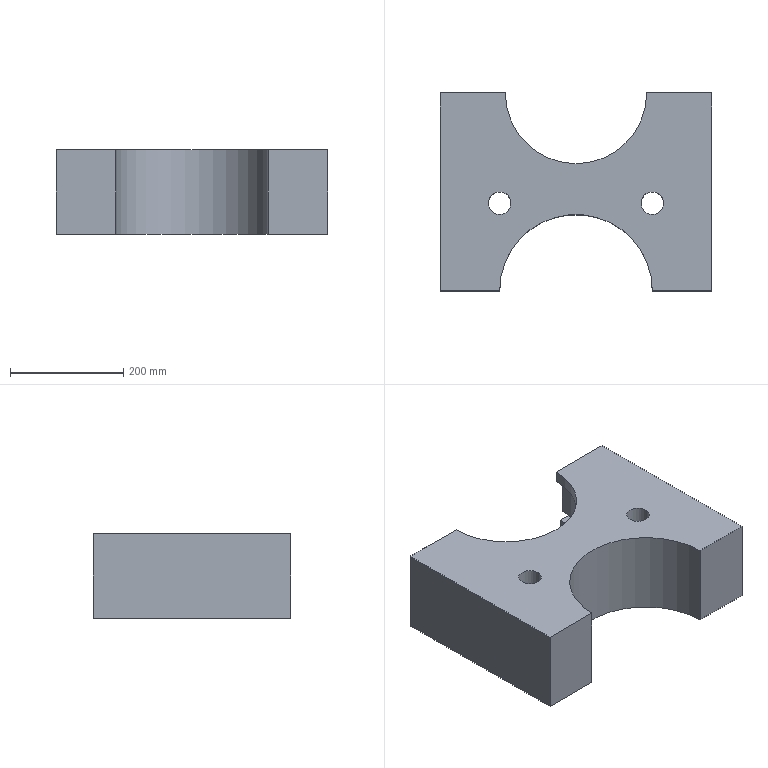Part | SolidWorks | features ICE 2, Extrusion 1, RevCut 1 | 1 solid | 20 faces | box 480 x 350 x 150 mm | volume 16005972 mm3 | plane 11 | cylinder 9 | commonest cylinder face diameters 40 x4 270 x2 250 x1 280 x1 310 x1
STEP:
#1=CARTESIAN_POINT('',(-155.,-20.,0.));
#2=VERTEX_POINT('',#1);
#3=CARTESIAN_POINT('',(-115.,-20.,0.));
#4=VERTEX_POINT('',#3);
#5=CARTESIAN_POINT('',(-135.,-20.,0.));
#6=DIRECTION('',(0.,0.,1.));
#7=DIRECTION('',(1.,0.,0.));
#8=AXIS2_PLACEMENT_3D('',#5,#6,#7);
#9=CIRCLE('',#8,20.);
#10=EDGE_CURVE('',#2,#4,#9,.T.);
#11=ORIENTED_EDGE('',*,*,#10,.F.);
#12=CARTESIAN_POINT('',(-155.,-20.,150.));
#13=VERTEX_POINT('',#12);
#14=CARTESIAN_POINT('',(-155.,-20.,0.));
#15=DIRECTION('',(0.,0.,1.));
#16=VECTOR('',#15,1000.);
#17=LINE('',#14,#16);
#18=EDGE_CURVE('',#2,#13,#17,.T.);
#19=ORIENTED_EDGE('',*,*,#18,.T.);
#20=CARTESIAN_POINT('',(-115.,-20.,150.));
#21=VERTEX_POINT('',#20);
#22=CARTESIAN_POINT('',(-135.,-20.,150.));
#23=DIRECTION('',(0.,0.,1.));
#24=DIRECTION('',(1.,0.,0.));
#25=AXIS2_PLACEMENT_3D('',#22,#23,#24);
#26=CIRCLE('',#25,20.);
#27=EDGE_CURVE('',#13,#21,#26,.T.);
#28=ORIENTED_EDGE('',*,*,#27,.T.);
#29=CARTESIAN_POINT('',(-115.,-20.,0.));
#30=DIRECTION('',(0.,0.,1.));
#31=VECTOR('',#30,1000.);
#32=LINE('',#29,#31);
#33=EDGE_CURVE('',#4,#21,#32,.T.);
#34=ORIENTED_EDGE('',*,*,#33,.F.);
#35=EDGE_LOOP('',(#11,#19,#28,#34));
#36=FACE_OUTER_BOUND('',#35,.T.);
#37=CARTESIAN_POINT('',(-135.,-20.,0.));
#38=DIRECTION('',(0.,0.,1.));
#39=DIRECTION('',(1.,0.,0.));
#40=AXIS2_PLACEMENT_3D('',#37,#38,#39);
#41=CYLINDRICAL_SURFACE('',#40,20.);
#42=ADVANCED_FACE('',(#36),#41,.F.);
#43=CARTESIAN_POINT('',(115.,-20.,0.));
#44=VERTEX_POINT('',#43);
#45=CARTESIAN_POINT('',(155.,-20.,0.));
#46=VERTEX_POINT('',#45);
#47=CARTESIAN_POINT('',(135.,-20.,0.));
#48=DIRECTION('',(0.,0.,1.));
#49=DIRECTION('',(-1.,0.,0.));
#50=AXIS2_PLACEMENT_3D('',#47,#48,#49);
#51=CIRCLE('',#50,20.);
#52=EDGE_CURVE('',#44,#46,#51,.T.);
#53=ORIENTED_EDGE('',*,*,#52,.F.);
#54=CARTESIAN_POINT('',(115.,-20.,150.));
#55=VERTEX_POINT('',#54);
#56=CARTESIAN_POINT('',(115.,-20.,0.));
#57=DIRECTION('',(0.,0.,1.));
#58=VECTOR('',#57,1000.);
#59=LINE('',#56,#58);
#60=EDGE_CURVE('',#44,#55,#59,.T.);
#61=ORIENTED_EDGE('',*,*,#60,.T.);
#62=CARTESIAN_POINT('',(155.,-20.,150.));
#63=VERTEX_POINT('',#62);
#64=CARTESIAN_POINT('',(135.,-20.,150.));
#65=DIRECTION('',(0.,0.,1.));
#66=DIRECTION('',(1.,0.,0.));
#67=AXIS2_PLACEMENT_3D('',#64,#65,#66);
#68=CIRCLE('',#67,20.);
#69=EDGE_CURVE('',#55,#63,#68,.T.);
#70=ORIENTED_EDGE('',*,*,#69,.T.);
#71=CARTESIAN_POINT('',(155.,-20.,0.));
#72=DIRECTION('',(0.,0.,1.));
#73=VECTOR('',#72,1000.);
#74=LINE('',#71,#73);
#75=EDGE_CURVE('',#46,#63,#74,.T.);
#76=ORIENTED_EDGE('',*,*,#75,.F.);
#77=EDGE_LOOP('',(#53,#61,#70,#76));
#78=FACE_OUTER_BOUND('',#77,.T.);
#79=CARTESIAN_POINT('',(135.,-20.,0.));
#80=DIRECTION('',(0.,0.,1.));
#81=DIRECTION('',(1.,0.,0.));
#82=AXIS2_PLACEMENT_3D('',#79,#80,#81);
#83=CYLINDRICAL_SURFACE('',#82,20.);
#84=ADVANCED_FACE('',(#78),#83,.F.);
#85=CARTESIAN_POINT('',(125.,175.,130.));
#86=VERTEX_POINT('',#85);
#87=CARTESIAN_POINT('',(140.,175.,130.));
#88=VERTEX_POINT('',#87);
#89=CARTESIAN_POINT('',(-240.,175.,130.));
#90=DIRECTION('',(1.,0.,0.));
#91=VECTOR('',#90,1000.);
#92=LINE('',#89,#91);
#93=EDGE_CURVE('',#86,#88,#92,.T.);
#94=ORIENTED_EDGE('',*,*,#93,.F.);
#95=CARTESIAN_POINT('',(125.,175.,150.));
#96=VERTEX_POINT('',#95);
#97=CARTESIAN_POINT('',(125.,175.,0.));
#98=DIRECTION('',(0.,0.,1.));
#99=VECTOR('',#98,1000.);
#100=LINE('',#97,#99);
#101=EDGE_CURVE('',#86,#96,#100,.T.);
#102=ORIENTED_EDGE('',*,*,#101,.T.);
#103=CARTESIAN_POINT('',(240.,175.,150.));
#104=VERTEX_POINT('',#103);
#105=CARTESIAN_POINT('',(-240.,175.,150.));
#106=DIRECTION('',(-1.,0.,0.));
#107=VECTOR('',#106,1000.);
#108=LINE('',#105,#107);
#109=EDGE_CURVE('',#104,#96,#108,.T.);
#110=ORIENTED_EDGE('',*,*,#109,.F.);
#111=CARTESIAN_POINT('',(240.,175.,0.));
#112=VERTEX_POINT('',#111);
#113=CARTESIAN_POINT('',(240.,175.,150.));
#114=DIRECTION('',(0.,0.,-1.));
#115=VECTOR('',#114,1000.);
#116=LINE('',#113,#115);
#117=EDGE_CURVE('',#104,#112,#116,.T.);
#118=ORIENTED_EDGE('',*,*,#117,.T.);
#119=CARTESIAN_POINT('',(135.,175.,0.));
#120=VERTEX_POINT('',#119);
#121=CARTESIAN_POINT('',(-240.,175.,0.));
#122=DIRECTION('',(-1.,0.,0.));
#123=VECTOR('',#122,1000.);
#124=LINE('',#121,#123);
#125=EDGE_CURVE('',#112,#120,#124,.T.);
#126=ORIENTED_EDGE('',*,*,#125,.T.);
#127=CARTESIAN_POINT('',(135.,175.,41.));
#128=VERTEX_POINT('',#127);
#129=CARTESIAN_POINT('',(135.,175.,150.));
#130=DIRECTION('',(0.,0.,-1.));
#131=VECTOR('',#130,1000.);
#132=LINE('',#129,#131);
#133=EDGE_CURVE('',#128,#120,#132,.T.);
#134=ORIENTED_EDGE('',*,*,#133,.F.);
#135=CARTESIAN_POINT('',(155.,175.,41.));
#136=VERTEX_POINT('',#135);
#137=CARTESIAN_POINT('',(-240.,175.,41.));
#138=DIRECTION('',(-1.,0.,0.));
#139=VECTOR('',#138,1000.);
#140=LINE('',#137,#139);
#141=EDGE_CURVE('',#136,#128,#140,.T.);
#142=ORIENTED_EDGE('',*,*,#141,.F.);
#143=CARTESIAN_POINT('',(155.,175.,58.));
#144=VERTEX_POINT('',#143);
#145=CARTESIAN_POINT('',(155.,175.,150.));
#146=DIRECTION('',(0.,0.,-1.));
#147=VECTOR('',#146,1000.);
#148=LINE('',#145,#147);
#149=EDGE_CURVE('',#144,#136,#148,.T.);
#150=ORIENTED_EDGE('',*,*,#149,.F.);
#151=CARTESIAN_POINT('',(140.,175.,58.));
#152=VERTEX_POINT('',#151);
#153=CARTESIAN_POINT('',(-240.,175.,58.));
#154=DIRECTION('',(1.,0.,0.));
#155=VECTOR('',#154,1000.);
#156=LINE('',#153,#155);
#157=EDGE_CURVE('',#152,#144,#156,.T.);
#158=ORIENTED_EDGE('',*,*,#157,.F.);
#159=CARTESIAN_POINT('',(140.,175.,150.));
#160=DIRECTION('',(0.,0.,-1.));
#161=VECTOR('',#160,1000.);
#162=LINE('',#159,#161);
#163=EDGE_CURVE('',#88,#152,#162,.T.);
#164=ORIENTED_EDGE('',*,*,#163,.F.);
#165=EDGE_LOOP('',(#94,#102,#110,#118,#126,#134,#142,#150,#158,#164));
#166=FACE_OUTER_BOUND('',#165,.T.);
#167=CARTESIAN_POINT('',(-240.,175.,150.));
#168=DIRECTION('',(0.,-1.,0.));
#169=DIRECTION('',(0.,0.,-1.));
#170=AXIS2_PLACEMENT_3D('',#167,#168,#169);
#171=PLANE('',#170);
#172=ADVANCED_FACE('',(#166),#171,.F.);
#173=CARTESIAN_POINT('',(-140.,175.,130.));
#174=VERTEX_POINT('',#173);
#175=CARTESIAN_POINT('',(-125.,175.,130.));
#176=VERTEX_POINT('',#175);
#177=CARTESIAN_POINT('',(-240.,175.,130.));
#178=DIRECTION('',(1.,0.,0.));
#179=VECTOR('',#178,1000.);
#180=LINE('',#177,#179);
#181=EDGE_CURVE('',#174,#176,#180,.T.);
#182=ORIENTED_EDGE('',*,*,#181,.F.);
#183=CARTESIAN_POINT('',(-140.,175.,58.));
#184=VERTEX_POINT('',#183);
#185=CARTESIAN_POINT('',(-140.,175.,150.));
#186=DIRECTION('',(0.,0.,1.));
#187=VECTOR('',#186,1000.);
#188=LINE('',#185,#187);
#189=EDGE_CURVE('',#184,#174,#188,.T.);
#190=ORIENTED_EDGE('',*,*,#189,.F.);
#191=CARTESIAN_POINT('',(-155.,175.,58.));
#192=VERTEX_POINT('',#191);
#193=CARTESIAN_POINT('',(-240.,175.,58.));
#194=DIRECTION('',(1.,0.,0.));
#195=VECTOR('',#194,1000.);
#196=LINE('',#193,#195);
#197=EDGE_CURVE('',#192,#184,#196,.T.);
#198=ORIENTED_EDGE('',*,*,#197,.F.);
#199=CARTESIAN_POINT('',(-155.,175.,41.));
#200=VERTEX_POINT('',#199);
#201=CARTESIAN_POINT('',(-155.,175.,150.));
#202=DIRECTION('',(0.,0.,1.));
#203=VECTOR('',#202,1000.);
#204=LINE('',#201,#203);
#205=EDGE_CURVE('',#200,#192,#204,.T.);
#206=ORIENTED_EDGE('',*,*,#205,.F.);
#207=CARTESIAN_POINT('',(-135.,175.,41.));
#208=VERTEX_POINT('',#207);
#209=CARTESIAN_POINT('',(-240.,175.,41.));
#210=DIRECTION('',(-1.,0.,0.));
#211=VECTOR('',#210,1000.);
#212=LINE('',#209,#211);
#213=EDGE_CURVE('',#208,#200,#212,.T.);
#214=ORIENTED_EDGE('',*,*,#213,.F.);
#215=CARTESIAN_POINT('',(-135.,175.,0.));
#216=VERTEX_POINT('',#215);
#217=CARTESIAN_POINT('',(-135.,175.,150.));
#218=DIRECTION('',(0.,0.,1.));
#219=VECTOR('',#218,1000.);
#220=LINE('',#217,#219);
#221=EDGE_CURVE('',#216,#208,#220,.T.);
#222=ORIENTED_EDGE('',*,*,#221,.F.);
#223=CARTESIAN_POINT('',(-240.,175.,0.));
#224=VERTEX_POINT('',#223);
#225=CARTESIAN_POINT('',(-240.,175.,0.));
#226=DIRECTION('',(-1.,0.,0.));
#227=VECTOR('',#226,1000.);
#228=LINE('',#225,#227);
#229=EDGE_CURVE('',#216,#224,#228,.T.);
#230=ORIENTED_EDGE('',*,*,#229,.T.);
#231=CARTESIAN_POINT('',(-240.,175.,150.));
#232=VERTEX_POINT('',#231);
#233=CARTESIAN_POINT('',(-240.,175.,150.));
#234=DIRECTION('',(0.,0.,-1.));
#235=VECTOR('',#234,1000.);
#236=LINE('',#233,#235);
#237=EDGE_CURVE('',#232,#224,#236,.T.);
#238=ORIENTED_EDGE('',*,*,#237,.F.);
#239=CARTESIAN_POINT('',(-125.,175.,150.));
#240=VERTEX_POINT('',#239);
#241=CARTESIAN_POINT('',(-240.,175.,150.));
#242=DIRECTION('',(-1.,0.,0.));
#243=VECTOR('',#242,1000.);
#244=LINE('',#241,#243);
#245=EDGE_CURVE('',#240,#232,#244,.T.);
#246=ORIENTED_EDGE('',*,*,#245,.F.);
#247=CARTESIAN_POINT('',(-125.,175.,0.));
#248=DIRECTION('',(0.,0.,-1.));
#249=VECTOR('',#248,1000.);
#250=LINE('',#247,#249);
#251=EDGE_CURVE('',#240,#176,#250,.T.);
#252=ORIENTED_EDGE('',*,*,#251,.T.);
#253=EDGE_LOOP('',(#182,#190,#198,#206,#214,#222,#230,#238,#246,#252));
#254=FACE_OUTER_BOUND('',#253,.T.);
#255=CARTESIAN_POINT('',(-240.,175.,150.));
#256=DIRECTION('',(0.,-1.,0.));
#257=DIRECTION('',(0.,0.,-1.));
#258=AXIS2_PLACEMENT_3D('',#255,#256,#257);
#259=PLANE('',#258);
#260=ADVANCED_FACE('',(#254),#259,.F.);
#261=CARTESIAN_POINT('',(0.,175.,130.));
#262=DIRECTION('',(0.,0.,1.));
#263=DIRECTION('',(-1.,0.,0.));
#264=AXIS2_PLACEMENT_3D('',#261,#262,#263);
#265=CIRCLE('',#264,125.);
#266=EDGE_CURVE('',#176,#86,#265,.T.);
#267=ORIENTED_EDGE('',*,*,#266,.F.);
#268=ORIENTED_EDGE('',*,*,#251,.F.);
#269=CARTESIAN_POINT('',(0.,175.,150.));
#270=DIRECTION('',(0.,0.,1.));
#271=DIRECTION('',(1.,0.,0.));
#272=AXIS2_PLACEMENT_3D('',#269,#270,#271);
#273=CIRCLE('',#272,125.);
#274=EDGE_CURVE('',#240,#96,#273,.T.);
#275=ORIENTED_EDGE('',*,*,#274,.T.);
#276=ORIENTED_EDGE('',*,*,#101,.F.);
#277=EDGE_LOOP('',(#267,#268,#275,#276));
#278=FACE_OUTER_BOUND('',#277,.T.);
#279=CARTESIAN_POINT('',(0.,175.,0.));
#280=DIRECTION('',(0.,0.,1.));
#281=DIRECTION('',(1.,0.,0.));
#282=AXIS2_PLACEMENT_3D('',#279,#280,#281);
#283=CYLINDRICAL_SURFACE('',#282,125.);
#284=ADVANCED_FACE('',(#278),#283,.F.);
#285=CARTESIAN_POINT('',(-240.,-175.,0.));
#286=VERTEX_POINT('',#285);
#287=CARTESIAN_POINT('',(-135.,-175.,0.));
#288=VERTEX_POINT('',#287);
#289=CARTESIAN_POINT('',(-240.,-175.,0.));
#290=DIRECTION('',(1.,0.,0.));
#291=VECTOR('',#290,1000.);
#292=LINE('',#289,#291);
#293=EDGE_CURVE('',#286,#288,#292,.T.);
#294=ORIENTED_EDGE('',*,*,#293,.T.);
#295=CARTESIAN_POINT('',(-135.,-175.,150.));
#296=VERTEX_POINT('',#295);
#297=CARTESIAN_POINT('',(-135.,-175.,0.));
#298=DIRECTION('',(0.,0.,1.));
#299=VECTOR('',#298,1000.);
#300=LINE('',#297,#299);
#301=EDGE_CURVE('',#288,#296,#300,.T.);
#302=ORIENTED_EDGE('',*,*,#301,.T.);
#303=CARTESIAN_POINT('',(-240.,-175.,150.));
#304=VERTEX_POINT('',#303);
#305=CARTESIAN_POINT('',(-240.,-175.,150.));
#306=DIRECTION('',(1.,0.,0.));
#307=VECTOR('',#306,1000.);
#308=LINE('',#305,#307);
#309=EDGE_CURVE('',#304,#296,#308,.T.);
#310=ORIENTED_EDGE('',*,*,#309,.F.);
#311=CARTESIAN_POINT('',(-240.,-175.,150.));
#312=DIRECTION('',(0.,0.,-1.));
#313=VECTOR('',#312,1000.);
#314=LINE('',#311,#313);
#315=EDGE_CURVE('',#304,#286,#314,.T.);
#316=ORIENTED_EDGE('',*,*,#315,.T.);
#317=EDGE_LOOP('',(#294,#302,#310,#316));
#318=FACE_OUTER_BOUND('',#317,.T.);
#319=CARTESIAN_POINT('',(-240.,-175.,150.));
#320=DIRECTION('',(0.,1.,0.));
#321=DIRECTION('',(0.,0.,1.));
#322=AXIS2_PLACEMENT_3D('',#319,#320,#321);
#323=PLANE('',#322);
#324=ADVANCED_FACE('',(#318),#323,.F.);
#325=CARTESIAN_POINT('',(240.,-175.,0.));
#326=VERTEX_POINT('',#325);
#327=CARTESIAN_POINT('',(240.,175.,0.));
#328=DIRECTION('',(0.,1.,0.));
#329=VECTOR('',#328,1000.);
#330=LINE('',#327,#329);
#331=EDGE_CURVE('',#326,#112,#330,.T.);
#332=ORIENTED_EDGE('',*,*,#331,.T.);
#333=ORIENTED_EDGE('',*,*,#117,.F.);
#334=CARTESIAN_POINT('',(240.,-175.,150.));
#335=VERTEX_POINT('',#334);
#336=CARTESIAN_POINT('',(240.,175.,150.));
#337=DIRECTION('',(0.,1.,0.));
#338=VECTOR('',#337,1000.);
#339=LINE('',#336,#338);
#340=EDGE_CURVE('',#335,#104,#339,.T.);
#341=ORIENTED_EDGE('',*,*,#340,.F.);
#342=CARTESIAN_POINT('',(240.,-175.,150.));
#343=DIRECTION('',(0.,0.,-1.));
#344=VECTOR('',#343,1000.);
#345=LINE('',#342,#344);
#346=EDGE_CURVE('',#335,#326,#345,.T.);
#347=ORIENTED_EDGE('',*,*,#346,.T.);
#348=EDGE_LOOP('',(#332,#333,#341,#347));
#349=FACE_OUTER_BOUND('',#348,.T.);
#350=CARTESIAN_POINT('',(240.,175.,150.));
#351=DIRECTION('',(-1.,0.,0.));
#352=DIRECTION('',(0.,-1.,0.));
#353=AXIS2_PLACEMENT_3D('',#350,#351,#352);
#354=PLANE('',#353);
#355=ADVANCED_FACE('',(#349),#354,.F.);
#356=CARTESIAN_POINT('',(-240.,175.,0.));
#357=DIRECTION('',(0.,-1.,0.));
#358=VECTOR('',#357,1000.);
#359=LINE('',#356,#358);
#360=EDGE_CURVE('',#224,#286,#359,.T.);
#361=ORIENTED_EDGE('',*,*,#360,.T.);
#362=ORIENTED_EDGE('',*,*,#315,.F.);
#363=CARTESIAN_POINT('',(-240.,175.,150.));
#364=DIRECTION('',(0.,-1.,0.));
#365=VECTOR('',#364,1000.);
#366=LINE('',#363,#365);
#367=EDGE_CURVE('',#232,#304,#366,.T.);
#368=ORIENTED_EDGE('',*,*,#367,.F.);
#369=ORIENTED_EDGE('',*,*,#237,.T.);
#370=EDGE_LOOP('',(#361,#362,#368,#369));
#371=FACE_OUTER_BOUND('',#370,.T.);
#372=CARTESIAN_POINT('',(-240.,175.,150.));
#373=DIRECTION('',(1.,0.,0.));
#374=DIRECTION('',(0.,1.,0.));
#375=AXIS2_PLACEMENT_3D('',#372,#373,#374);
#376=PLANE('',#375);
#377=ADVANCED_FACE('',(#371),#376,.F.);
#378=CARTESIAN_POINT('',(135.,-175.,150.));
#379=VERTEX_POINT('',#378);
#380=CARTESIAN_POINT('',(-240.,-175.,150.));
#381=DIRECTION('',(1.,0.,0.));
#382=VECTOR('',#381,1000.);
#383=LINE('',#380,#382);
#384=EDGE_CURVE('',#379,#335,#383,.T.);
#385=ORIENTED_EDGE('',*,*,#384,.F.);
#386=CARTESIAN_POINT('',(135.,-175.,0.));
#387=VERTEX_POINT('',#386);
#388=CARTESIAN_POINT('',(135.,-175.,0.));
#389=DIRECTION('',(0.,0.,-1.));
#390=VECTOR('',#389,1000.);
#391=LINE('',#388,#390);
#392=EDGE_CURVE('',#379,#387,#391,.T.);
#393=ORIENTED_EDGE('',*,*,#392,.T.);
#394=CARTESIAN_POINT('',(-240.,-175.,0.));
#395=DIRECTION('',(1.,0.,0.));
#396=VECTOR('',#395,1000.);
#397=LINE('',#394,#396);
#398=EDGE_CURVE('',#387,#326,#397,.T.);
#399=ORIENTED_EDGE('',*,*,#398,.T.);
#400=ORIENTED_EDGE('',*,*,#346,.F.);
#401=EDGE_LOOP('',(#385,#393,#399,#400));
#402=FACE_OUTER_BOUND('',#401,.T.);
#403=CARTESIAN_POINT('',(-240.,-175.,150.));
#404=DIRECTION('',(0.,1.,0.));
#405=DIRECTION('',(0.,0.,1.));
#406=AXIS2_PLACEMENT_3D('',#403,#404,#405);
#407=PLANE('',#406);
#408=ADVANCED_FACE('',(#402),#407,.F.);
#409=CARTESIAN_POINT('',(0.,-175.,150.));
#410=DIRECTION('',(0.,0.,1.));
#411=DIRECTION('',(1.,0.,0.));
#412=AXIS2_PLACEMENT_3D('',#409,#410,#411);
#413=CIRCLE('',#412,135.);
#414=EDGE_CURVE('',#379,#296,#413,.T.);
#415=ORIENTED_EDGE('',*,*,#414,.F.);
#416=ORIENTED_EDGE('',*,*,#384,.T.);
#417=ORIENTED_EDGE('',*,*,#340,.T.);
#418=ORIENTED_EDGE('',*,*,#109,.T.);
#419=ORIENTED_EDGE('',*,*,#274,.F.);
#420=ORIENTED_EDGE('',*,*,#245,.T.);
#421=ORIENTED_EDGE('',*,*,#367,.T.);
#422=ORIENTED_EDGE('',*,*,#309,.T.);
#423=EDGE_LOOP('',(#415,#416,#417,#418,#419,#420,#421,#422));
#424=FACE_OUTER_BOUND('',#423,.T.);
#425=CARTESIAN_POINT('',(-135.,-20.,150.));
#426=DIRECTION('',(0.,0.,1.));
#427=DIRECTION('',(1.,0.,0.));
#428=AXIS2_PLACEMENT_3D('',#425,#426,#427);
#429=CIRCLE('',#428,20.);
#430=EDGE_CURVE('',#21,#13,#429,.T.);
#431=ORIENTED_EDGE('',*,*,#430,.F.);
#432=ORIENTED_EDGE('',*,*,#27,.F.);
#433=EDGE_LOOP('',(#431,#432));
#434=FACE_BOUND('',#433,.T.);
#435=CARTESIAN_POINT('',(135.,-20.,150.));
#436=DIRECTION('',(0.,0.,1.));
#437=DIRECTION('',(1.,0.,0.));
#438=AXIS2_PLACEMENT_3D('',#435,#436,#437);
#439=CIRCLE('',#438,20.);
#440=EDGE_CURVE('',#63,#55,#439,.T.);
#441=ORIENTED_EDGE('',*,*,#440,.F.);
#442=ORIENTED_EDGE('',*,*,#69,.F.);
#443=EDGE_LOOP('',(#441,#442));
#444=FACE_BOUND('',#443,.T.);
#445=CARTESIAN_POINT('',(0.,0.,150.));
#446=DIRECTION('',(0.,0.,1.));
#447=DIRECTION('',(1.,0.,0.));
#448=AXIS2_PLACEMENT_3D('',#445,#446,#447);
#449=PLANE('',#448);
#450=ADVANCED_FACE('',(#424,#434,#444),#449,.T.);
#451=CARTESIAN_POINT('',(0.,175.,0.));
#452=DIRECTION('',(0.,0.,1.));
#453=DIRECTION('',(1.,0.,0.));
#454=AXIS2_PLACEMENT_3D('',#451,#452,#453);
#455=CIRCLE('',#454,135.);
#456=EDGE_CURVE('',#216,#120,#455,.T.);
#457=ORIENTED_EDGE('',*,*,#456,.T.);
#458=ORIENTED_EDGE('',*,*,#125,.F.);
#459=ORIENTED_EDGE('',*,*,#331,.F.);
#460=ORIENTED_EDGE('',*,*,#398,.F.);
#461=CARTESIAN_POINT('',(0.,-175.,0.));
#462=DIRECTION('',(0.,0.,1.));
#463=DIRECTION('',(1.,0.,0.));
#464=AXIS2_PLACEMENT_3D('',#461,#462,#463);
#465=CIRCLE('',#464,135.);
#466=EDGE_CURVE('',#387,#288,#465,.T.);
#467=ORIENTED_EDGE('',*,*,#466,.T.);
#468=ORIENTED_EDGE('',*,*,#293,.F.);
#469=ORIENTED_EDGE('',*,*,#360,.F.);
#470=ORIENTED_EDGE('',*,*,#229,.F.);
#471=EDGE_LOOP('',(#457,#458,#459,#460,#467,#468,#469,#470));
#472=FACE_OUTER_BOUND('',#471,.T.);
#473=CARTESIAN_POINT('',(-135.,-20.,0.));
#474=DIRECTION('',(0.,0.,1.));
#475=DIRECTION('',(1.,0.,0.));
#476=AXIS2_PLACEMENT_3D('',#473,#474,#475);
#477=CIRCLE('',#476,20.);
#478=EDGE_CURVE('',#4,#2,#477,.T.);
#479=ORIENTED_EDGE('',*,*,#478,.T.);
#480=ORIENTED_EDGE('',*,*,#10,.T.);
#481=EDGE_LOOP('',(#479,#480));
#482=FACE_BOUND('',#481,.T.);
#483=CARTESIAN_POINT('',(135.,-20.,0.));
#484=DIRECTION('',(0.,0.,1.));
#485=DIRECTION('',(-1.,0.,0.));
#486=AXIS2_PLACEMENT_3D('',#483,#484,#485);
#487=CIRCLE('',#486,20.);
#488=EDGE_CURVE('',#46,#44,#487,.T.);
#489=ORIENTED_EDGE('',*,*,#488,.T.);
#490=ORIENTED_EDGE('',*,*,#52,.T.);
#491=EDGE_LOOP('',(#489,#490));
#492=FACE_BOUND('',#491,.T.);
#493=CARTESIAN_POINT('',(0.,0.,0.));
#494=DIRECTION('',(0.,0.,1.));
#495=DIRECTION('',(1.,0.,0.));
#496=AXIS2_PLACEMENT_3D('',#493,#494,#495);
#497=PLANE('',#496);
#498=ADVANCED_FACE('',(#472,#482,#492),#497,.F.);
#499=ORIENTED_EDGE('',*,*,#60,.F.);
#500=ORIENTED_EDGE('',*,*,#488,.F.);
#501=ORIENTED_EDGE('',*,*,#75,.T.);
#502=ORIENTED_EDGE('',*,*,#440,.T.);
#503=EDGE_LOOP('',(#499,#500,#501,#502));
#504=FACE_OUTER_BOUND('',#503,.T.);
#505=CARTESIAN_POINT('',(135.,-20.,0.));
#506=DIRECTION('',(0.,0.,1.));
#507=DIRECTION('',(1.,0.,0.));
#508=AXIS2_PLACEMENT_3D('',#505,#506,#507);
#509=CYLINDRICAL_SURFACE('',#508,20.);
#510=ADVANCED_FACE('',(#504),#509,.F.);
#511=ORIENTED_EDGE('',*,*,#18,.F.);
#512=ORIENTED_EDGE('',*,*,#478,.F.);
#513=ORIENTED_EDGE('',*,*,#33,.T.);
#514=ORIENTED_EDGE('',*,*,#430,.T.);
#515=EDGE_LOOP('',(#511,#512,#513,#514));
#516=FACE_OUTER_BOUND('',#515,.T.);
#517=CARTESIAN_POINT('',(-135.,-20.,0.));
#518=DIRECTION('',(0.,0.,1.));
#519=DIRECTION('',(1.,0.,0.));
#520=AXIS2_PLACEMENT_3D('',#517,#518,#519);
#521=CYLINDRICAL_SURFACE('',#520,20.);
#522=ADVANCED_FACE('',(#516),#521,.F.);
#523=ORIENTED_EDGE('',*,*,#466,.F.);
#524=ORIENTED_EDGE('',*,*,#392,.F.);
#525=ORIENTED_EDGE('',*,*,#414,.T.);
#526=ORIENTED_EDGE('',*,*,#301,.F.);
#527=EDGE_LOOP('',(#523,#524,#525,#526));
#528=FACE_OUTER_BOUND('',#527,.T.);
#529=CARTESIAN_POINT('',(0.,-175.,0.));
#530=DIRECTION('',(0.,0.,1.));
#531=DIRECTION('',(1.,0.,0.));
#532=AXIS2_PLACEMENT_3D('',#529,#530,#531);
#533=CYLINDRICAL_SURFACE('',#532,135.);
#534=ADVANCED_FACE('',(#528),#533,.F.);
#535=ORIENTED_EDGE('',*,*,#163,.T.);
#536=CARTESIAN_POINT('',(0.,175.,58.));
#537=DIRECTION('',(0.,0.,1.));
#538=DIRECTION('',(1.,0.,0.));
#539=AXIS2_PLACEMENT_3D('',#536,#537,#538);
#540=CIRCLE('',#539,140.);
#541=EDGE_CURVE('',#184,#152,#540,.T.);
#542=ORIENTED_EDGE('',*,*,#541,.F.);
#543=ORIENTED_EDGE('',*,*,#189,.T.);
#544=CARTESIAN_POINT('',(0.,175.,130.));
#545=DIRECTION('',(0.,0.,1.));
#546=DIRECTION('',(1.,0.,0.));
#547=AXIS2_PLACEMENT_3D('',#544,#545,#546);
#548=CIRCLE('',#547,140.);
#549=EDGE_CURVE('',#174,#88,#548,.T.);
#550=ORIENTED_EDGE('',*,*,#549,.T.);
#551=EDGE_LOOP('',(#535,#542,#543,#550));
#552=FACE_OUTER_BOUND('',#551,.T.);
#553=CARTESIAN_POINT('',(0.,175.,150.));
#554=DIRECTION('',(0.,0.,1.));
#555=DIRECTION('',(1.,0.,0.));
#556=AXIS2_PLACEMENT_3D('',#553,#554,#555);
#557=CYLINDRICAL_SURFACE('',#556,140.);
#558=ADVANCED_FACE('',(#552),#557,.F.);
#559=ORIENTED_EDGE('',*,*,#157,.T.);
#560=CARTESIAN_POINT('',(0.,175.,58.));
#561=DIRECTION('',(0.,0.,1.));
#562=DIRECTION('',(1.,0.,0.));
#563=AXIS2_PLACEMENT_3D('',#560,#561,#562);
#564=CIRCLE('',#563,155.);
#565=EDGE_CURVE('',#192,#144,#564,.T.);
#566=ORIENTED_EDGE('',*,*,#565,.F.);
#567=ORIENTED_EDGE('',*,*,#197,.T.);
#568=ORIENTED_EDGE('',*,*,#541,.T.);
#569=EDGE_LOOP('',(#559,#566,#567,#568));
#570=FACE_OUTER_BOUND('',#569,.T.);
#571=CARTESIAN_POINT('',(-140.,175.,58.));
#572=DIRECTION('',(0.,0.,-1.));
#573=DIRECTION('',(-1.,0.,0.));
#574=AXIS2_PLACEMENT_3D('',#571,#572,#573);
#575=PLANE('',#574);
#576=ADVANCED_FACE('',(#570),#575,.T.);
#577=ORIENTED_EDGE('',*,*,#149,.T.);
#578=CARTESIAN_POINT('',(0.,175.,41.));
#579=DIRECTION('',(0.,0.,1.));
#580=DIRECTION('',(1.,0.,0.));
#581=AXIS2_PLACEMENT_3D('',#578,#579,#580);
#582=CIRCLE('',#581,155.);
#583=EDGE_CURVE('',#200,#136,#582,.T.);
#584=ORIENTED_EDGE('',*,*,#583,.F.);
#585=ORIENTED_EDGE('',*,*,#205,.T.);
#586=ORIENTED_EDGE('',*,*,#565,.T.);
#587=EDGE_LOOP('',(#577,#584,#585,#586));
#588=FACE_OUTER_BOUND('',#587,.T.);
#589=CARTESIAN_POINT('',(0.,175.,150.));
#590=DIRECTION('',(0.,0.,1.));
#591=DIRECTION('',(1.,0.,0.));
#592=AXIS2_PLACEMENT_3D('',#589,#590,#591);
#593=CYLINDRICAL_SURFACE('',#592,155.);
#594=ADVANCED_FACE('',(#588),#593,.F.);
#595=ORIENTED_EDGE('',*,*,#141,.T.);
#596=CARTESIAN_POINT('',(0.,175.,41.));
#597=DIRECTION('',(0.,0.,1.));
#598=DIRECTION('',(1.,0.,0.));
#599=AXIS2_PLACEMENT_3D('',#596,#597,#598);
#600=CIRCLE('',#599,135.);
#601=EDGE_CURVE('',#208,#128,#600,.T.);
#602=ORIENTED_EDGE('',*,*,#601,.F.);
#603=ORIENTED_EDGE('',*,*,#213,.T.);
#604=ORIENTED_EDGE('',*,*,#583,.T.);
#605=EDGE_LOOP('',(#595,#602,#603,#604));
#606=FACE_OUTER_BOUND('',#605,.T.);
#607=CARTESIAN_POINT('',(-155.,175.,41.));
#608=DIRECTION('',(0.,0.,1.));
#609=DIRECTION('',(1.,0.,0.));
#610=AXIS2_PLACEMENT_3D('',#607,#608,#609);
#611=PLANE('',#610);
#612=ADVANCED_FACE('',(#606),#611,.T.);
#613=ORIENTED_EDGE('',*,*,#133,.T.);
#614=ORIENTED_EDGE('',*,*,#456,.F.);
#615=ORIENTED_EDGE('',*,*,#221,.T.);
#616=ORIENTED_EDGE('',*,*,#601,.T.);
#617=EDGE_LOOP('',(#613,#614,#615,#616));
#618=FACE_OUTER_BOUND('',#617,.T.);
#619=CARTESIAN_POINT('',(0.,175.,150.));
#620=DIRECTION('',(0.,0.,1.));
#621=DIRECTION('',(1.,0.,0.));
#622=AXIS2_PLACEMENT_3D('',#619,#620,#621);
#623=CYLINDRICAL_SURFACE('',#622,135.);
#624=ADVANCED_FACE('',(#618),#623,.F.);
#625=ORIENTED_EDGE('',*,*,#93,.T.);
#626=ORIENTED_EDGE('',*,*,#549,.F.);
#627=ORIENTED_EDGE('',*,*,#181,.T.);
#628=ORIENTED_EDGE('',*,*,#266,.T.);
#629=EDGE_LOOP('',(#625,#626,#627,#628));
#630=FACE_OUTER_BOUND('',#629,.T.);
#631=CARTESIAN_POINT('',(0.,175.,130.));
#632=DIRECTION('',(0.,0.,-1.));
#633=DIRECTION('',(-1.,0.,0.));
#634=AXIS2_PLACEMENT_3D('',#631,#632,#633);
#635=PLANE('',#634);
#636=ADVANCED_FACE('',(#630),#635,.T.);
#637=CLOSED_SHELL('',(#42,#84,#172,#260,#284,#324,#355,#377,#408,#450,#498,#510,#522,#534,#558,#576,#594,#612,#624,#636));
#638=MANIFOLD_SOLID_BREP('',#637);
#639=CARTESIAN_POINT('',(0.,0.,0.));
#640=DIRECTION('',(0.,0.,1.));
#641=DIRECTION('',(1.,0.,0.));
#642=AXIS2_PLACEMENT_3D('',#639,#640,#641);
#643=(LENGTH_UNIT()NAMED_UNIT(*)SI_UNIT(.MILLI.,.METRE.));
#644=UNCERTAINTY_MEASURE_WITH_UNIT(LENGTH_MEASURE(0.00001),#643,'','');
#645=(NAMED_UNIT(*)PLANE_ANGLE_UNIT()SI_UNIT($,.RADIAN.));
#646=(NAMED_UNIT(*)SI_UNIT($,.STERADIAN.)SOLID_ANGLE_UNIT());
#647=(GEOMETRIC_REPRESENTATION_CONTEXT(3)GLOBAL_UNCERTAINTY_ASSIGNED_CONTEXT((#644))GLOBAL_UNIT_ASSIGNED_CONTEXT((#643,#645,#646))REPRESENTATION_CONTEXT('',''));
#648=ADVANCED_BREP_SHAPE_REPRESENTATION('',(#638,#642),#647);